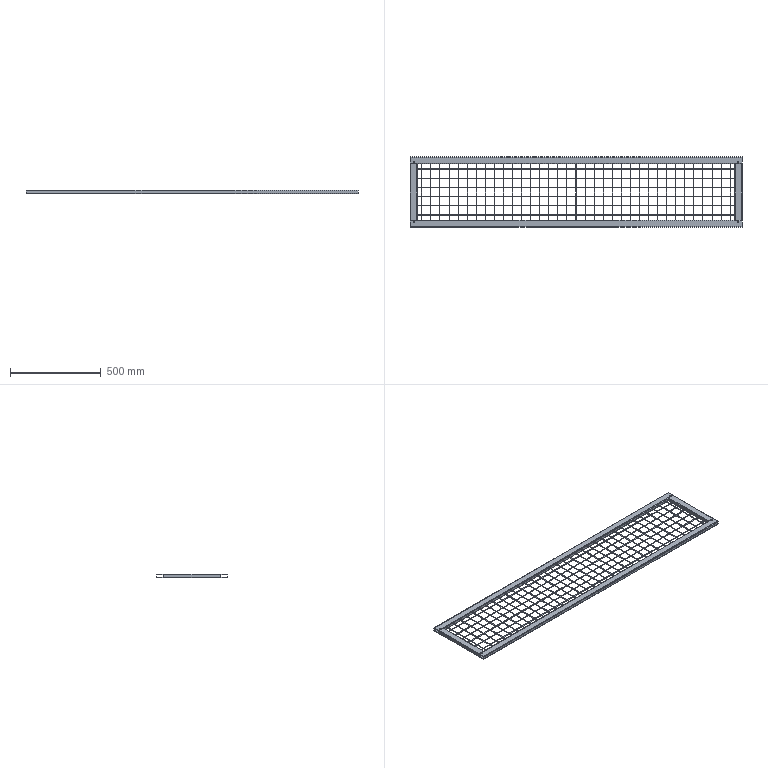Part | SolidWorks | features BaseBody 45 | 45 solids | 244 faces | box 1830 x 390 x 20 mm | volume 1182767 mm3 | cylinder 122 | plane 122 | commonest cylinder face diameters 4 x98 8 x16 5 x8